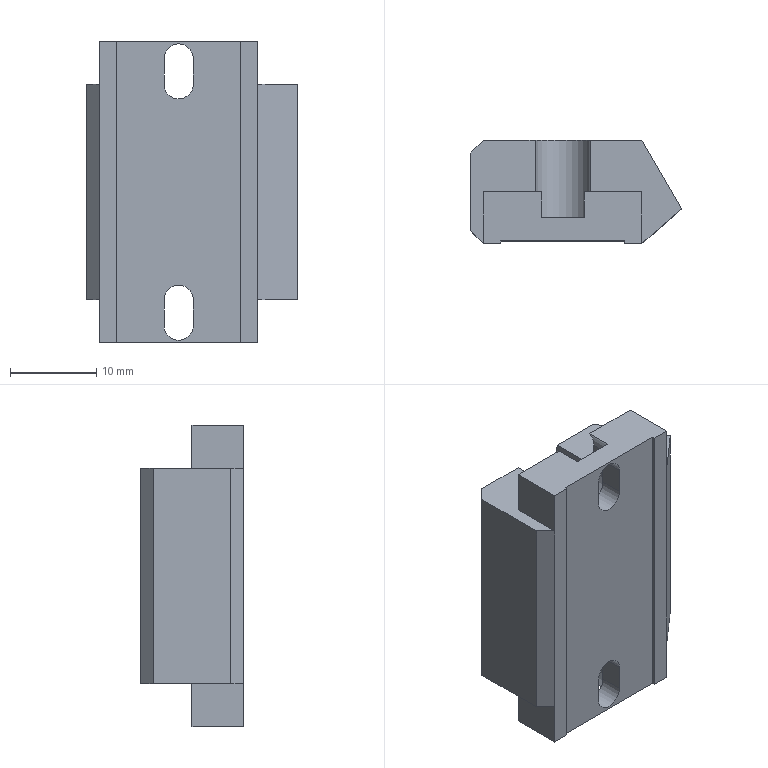Part | SolidWorks | features ICE 10, Chamfer 1, Extrusion 1 | 1 solid | 60 faces | box 24.5 x 12 x 35 mm | volume 6825 mm3 | plane 39 | cylinder 21 | commonest cylinder face diameters 6.4 x7 3.4 x6 2 x4 4 x4